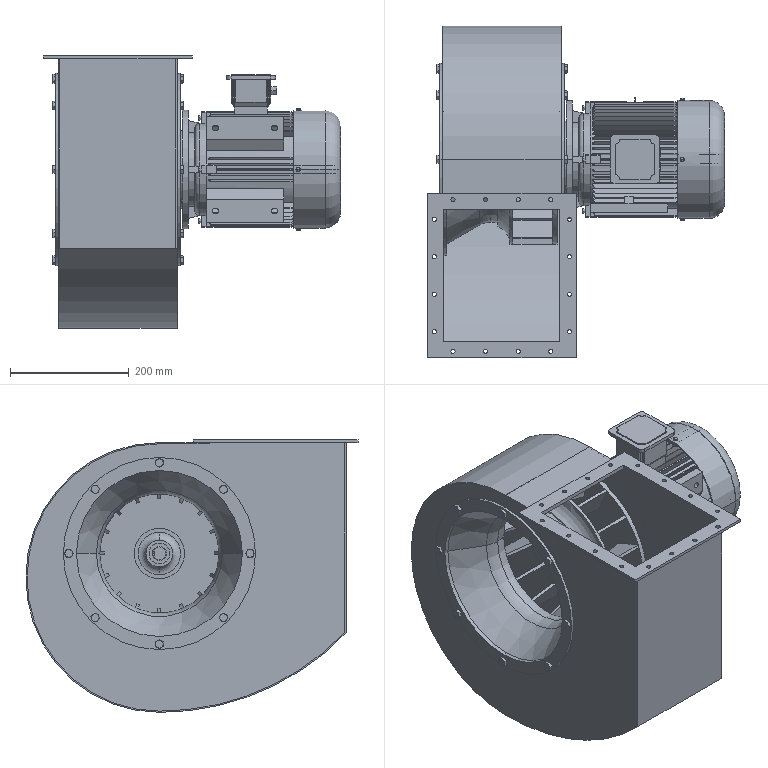Part | SolidWorks | 3 solids | 1099 faces | box 501 x 560.054 x 460 mm | volume 9683127 mm3 | plane 638 | cone 236 | cylinder 189 | torus 28 | sphere 8 | commonest cylinder face diameters 7 x32 74.4 x32 3.937 x10 171 x10 5.5 x9 6.7 x8